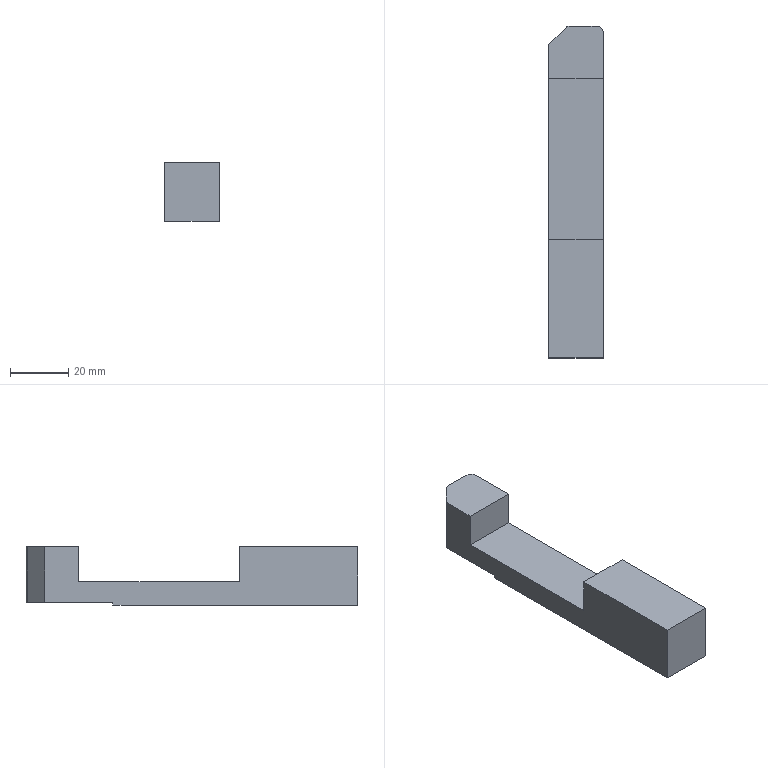Part | NX | features 20 2 | 1 solid | 15 faces | box 18.5 x 113.5 x 20 mm | volume 28823 mm3 | plane 13 | cylinder 2 | commonest cylinder face diameters 4 x2
STEP:
#1=CARTESIAN_POINT('',(316.699,-435.5,4.5));
#2=VERTEX_POINT('',#1);
#3=CARTESIAN_POINT('',(316.699,-490.5,4.5));
#4=VERTEX_POINT('',#3);
#5=CARTESIAN_POINT('',(316.699,-483.5,4.5));
#6=DIRECTION('',(0.,-1.,0.));
#7=VECTOR('',#6,1000.);
#8=LINE('',#5,#7);
#9=EDGE_CURVE('',#2,#4,#8,.T.);
#10=ORIENTED_EDGE('',*,*,#9,.T.);
#11=CARTESIAN_POINT('',(335.199,-490.5,4.5));
#12=VERTEX_POINT('',#11);
#13=CARTESIAN_POINT('',(297.899,-490.5,4.5));
#14=DIRECTION('',(-1.,0.,0.));
#15=VECTOR('',#14,1000.);
#16=LINE('',#13,#15);
#17=EDGE_CURVE('',#12,#4,#16,.T.);
#18=ORIENTED_EDGE('',*,*,#17,.F.);
#19=CARTESIAN_POINT('',(335.199,-435.5,4.5));
#20=VERTEX_POINT('',#19);
#21=CARTESIAN_POINT('',(335.199,-419.,4.5));
#22=DIRECTION('',(0.,1.,0.));
#23=VECTOR('',#22,1000.);
#24=LINE('',#21,#23);
#25=EDGE_CURVE('',#12,#20,#24,.T.);
#26=ORIENTED_EDGE('',*,*,#25,.T.);
#27=CARTESIAN_POINT('',(320.299,-435.5,4.5));
#28=DIRECTION('',(-1.,0.,0.));
#29=VECTOR('',#28,1000.);
#30=LINE('',#27,#29);
#31=EDGE_CURVE('',#20,#2,#30,.T.);
#32=ORIENTED_EDGE('',*,*,#31,.T.);
#33=EDGE_LOOP('',(#10,#18,#26,#32));
#34=FACE_BOUND('',#33,.T.);
#35=CARTESIAN_POINT('',(296.899,-343.,4.5));
#36=DIRECTION('',(0.,0.,1.));
#37=DIRECTION('',(1.,0.,0.));
#38=AXIS2_PLACEMENT_3D('',#35,#36,#37);
#39=PLANE('',#38);
#40=ADVANCED_FACE('',(#34),#39,.T.);
#41=CARTESIAN_POINT('',(316.699,-447.223,-2.5));
#42=VERTEX_POINT('',#41);
#43=CARTESIAN_POINT('',(316.699,-423.94,-2.5));
#44=VERTEX_POINT('',#43);
#45=CARTESIAN_POINT('',(316.699,-483.5,-2.5));
#46=DIRECTION('',(0.,1.,0.));
#47=VECTOR('',#46,1000.);
#48=LINE('',#45,#47);
#49=EDGE_CURVE('',#42,#44,#48,.T.);
#50=ORIENTED_EDGE('',*,*,#49,.F.);
#51=CARTESIAN_POINT('',(316.699,-447.223,-3.5));
#52=VERTEX_POINT('',#51);
#53=CARTESIAN_POINT('',(316.699,-447.223,-3.5));
#54=DIRECTION('',(0.,0.,1.));
#55=VECTOR('',#54,1000.);
#56=LINE('',#53,#55);
#57=EDGE_CURVE('',#52,#42,#56,.T.);
#58=ORIENTED_EDGE('',*,*,#57,.F.);
#59=CARTESIAN_POINT('',(316.699,-531.,-3.5));
#60=VERTEX_POINT('',#59);
#61=CARTESIAN_POINT('',(316.699,-483.5,-3.5));
#62=DIRECTION('',(0.,1.,0.));
#63=VECTOR('',#62,1000.);
#64=LINE('',#61,#63);
#65=EDGE_CURVE('',#60,#52,#64,.T.);
#66=ORIENTED_EDGE('',*,*,#65,.F.);
#67=CARTESIAN_POINT('',(316.699,-531.,16.5));
#68=VERTEX_POINT('',#67);
#69=CARTESIAN_POINT('',(316.699,-531.,-3.5));
#70=DIRECTION('',(0.,0.,1.));
#71=VECTOR('',#70,1000.);
#72=LINE('',#69,#71);
#73=EDGE_CURVE('',#60,#68,#72,.T.);
#74=ORIENTED_EDGE('',*,*,#73,.T.);
#75=CARTESIAN_POINT('',(316.699,-490.5,16.5));
#76=VERTEX_POINT('',#75);
#77=CARTESIAN_POINT('',(316.699,-453.,16.5));
#78=DIRECTION('',(0.,1.,0.));
#79=VECTOR('',#78,1000.);
#80=LINE('',#77,#79);
#81=EDGE_CURVE('',#68,#76,#80,.T.);
#82=ORIENTED_EDGE('',*,*,#81,.T.);
#83=CARTESIAN_POINT('',(316.699,-490.5,-3.5));
#84=DIRECTION('',(0.,0.,-1.));
#85=VECTOR('',#84,1000.);
#86=LINE('',#83,#85);
#87=EDGE_CURVE('',#76,#4,#86,.T.);
#88=ORIENTED_EDGE('',*,*,#87,.T.);
#89=ORIENTED_EDGE('',*,*,#9,.F.);
#90=CARTESIAN_POINT('',(316.699,-435.5,16.5));
#91=VERTEX_POINT('',#90);
#92=CARTESIAN_POINT('',(316.699,-435.5,22.5));
#93=DIRECTION('',(0.,0.,1.));
#94=VECTOR('',#93,1000.);
#95=LINE('',#92,#94);
#96=EDGE_CURVE('',#2,#91,#95,.T.);
#97=ORIENTED_EDGE('',*,*,#96,.T.);
#98=CARTESIAN_POINT('',(316.699,-423.94,16.5));
#99=VERTEX_POINT('',#98);
#100=CARTESIAN_POINT('',(316.699,-468.,16.5));
#101=DIRECTION('',(0.,1.,0.));
#102=VECTOR('',#101,1000.);
#103=LINE('',#100,#102);
#104=EDGE_CURVE('',#91,#99,#103,.T.);
#105=ORIENTED_EDGE('',*,*,#104,.T.);
#106=CARTESIAN_POINT('',(316.699,-423.94,-2.));
#107=DIRECTION('',(0.,0.,1.));
#108=VECTOR('',#107,1000.);
#109=LINE('',#106,#108);
#110=EDGE_CURVE('',#44,#99,#109,.T.);
#111=ORIENTED_EDGE('',*,*,#110,.F.);
#112=EDGE_LOOP('',(#50,#58,#66,#74,#82,#88,#89,#97,#105,#111));
#113=FACE_BOUND('',#112,.T.);
#114=CARTESIAN_POINT('',(316.699,-483.5,-3.5));
#115=DIRECTION('',(1.,0.,0.));
#116=DIRECTION('',(0.,1.,0.));
#117=AXIS2_PLACEMENT_3D('',#114,#115,#116);
#118=PLANE('',#117);
#119=ADVANCED_FACE('',(#113),#118,.F.);
#120=CARTESIAN_POINT('',(335.199,-447.223,-2.5));
#121=VERTEX_POINT('',#120);
#122=CARTESIAN_POINT('',(433.109,-447.223,-2.5));
#123=DIRECTION('',(-1.,0.,0.));
#124=VECTOR('',#123,1000.);
#125=LINE('',#122,#124);
#126=EDGE_CURVE('',#121,#42,#125,.T.);
#127=ORIENTED_EDGE('',*,*,#126,.T.);
#128=ORIENTED_EDGE('',*,*,#49,.T.);
#129=CARTESIAN_POINT('',(322.553,-418.086,-2.5));
#130=VERTEX_POINT('',#129);
#131=CARTESIAN_POINT('',(320.376,-420.263,-2.5));
#132=DIRECTION('',(0.7071,0.7071,0.));
#133=VECTOR('',#132,1000.);
#134=LINE('',#131,#133);
#135=EDGE_CURVE('',#44,#130,#134,.T.);
#136=ORIENTED_EDGE('',*,*,#135,.T.);
#137=CARTESIAN_POINT('',(323.967,-417.5,-2.5));
#138=VERTEX_POINT('',#137);
#139=CARTESIAN_POINT('',(323.967,-419.5,-2.5));
#140=DIRECTION('',(0.,0.,-1.));
#141=DIRECTION('',(-1.,0.,0.));
#142=AXIS2_PLACEMENT_3D('',#139,#140,#141);
#143=CIRCLE('',#142,2.);
#144=EDGE_CURVE('',#130,#138,#143,.T.);
#145=ORIENTED_EDGE('',*,*,#144,.T.);
#146=CARTESIAN_POINT('',(333.199,-417.5,-2.5));
#147=VERTEX_POINT('',#146);
#148=CARTESIAN_POINT('',(325.199,-417.5,-2.5));
#149=DIRECTION('',(1.,0.,0.));
#150=VECTOR('',#149,1000.);
#151=LINE('',#148,#150);
#152=EDGE_CURVE('',#138,#147,#151,.T.);
#153=ORIENTED_EDGE('',*,*,#152,.T.);
#154=CARTESIAN_POINT('',(335.199,-419.5,-2.5));
#155=VERTEX_POINT('',#154);
#156=CARTESIAN_POINT('',(333.199,-419.5,-2.5));
#157=DIRECTION('',(0.,0.,-1.));
#158=DIRECTION('',(-1.,0.,0.));
#159=AXIS2_PLACEMENT_3D('',#156,#157,#158);
#160=CIRCLE('',#159,2.);
#161=EDGE_CURVE('',#147,#155,#160,.T.);
#162=ORIENTED_EDGE('',*,*,#161,.T.);
#163=CARTESIAN_POINT('',(335.199,-419.,-2.5));
#164=DIRECTION('',(0.,-1.,0.));
#165=VECTOR('',#164,1000.);
#166=LINE('',#163,#165);
#167=EDGE_CURVE('',#155,#121,#166,.T.);
#168=ORIENTED_EDGE('',*,*,#167,.T.);
#169=EDGE_LOOP('',(#127,#128,#136,#145,#153,#162,#168));
#170=FACE_BOUND('',#169,.T.);
#171=CARTESIAN_POINT('',(325.199,-419.,-2.5));
#172=DIRECTION('',(0.,0.,-1.));
#173=DIRECTION('',(-1.,0.,0.));
#174=AXIS2_PLACEMENT_3D('',#171,#172,#173);
#175=PLANE('',#174);
#176=ADVANCED_FACE('',(#170),#175,.T.);
#177=ORIENTED_EDGE('',*,*,#25,.F.);
#178=CARTESIAN_POINT('',(335.199,-490.5,16.5));
#179=VERTEX_POINT('',#178);
#180=CARTESIAN_POINT('',(335.199,-490.5,-3.5));
#181=DIRECTION('',(0.,0.,1.));
#182=VECTOR('',#181,1000.);
#183=LINE('',#180,#182);
#184=EDGE_CURVE('',#12,#179,#183,.T.);
#185=ORIENTED_EDGE('',*,*,#184,.T.);
#186=CARTESIAN_POINT('',(335.199,-531.,16.5));
#187=VERTEX_POINT('',#186);
#188=CARTESIAN_POINT('',(335.199,-453.,16.5));
#189=DIRECTION('',(0.,-1.,0.));
#190=VECTOR('',#189,1000.);
#191=LINE('',#188,#190);
#192=EDGE_CURVE('',#179,#187,#191,.T.);
#193=ORIENTED_EDGE('',*,*,#192,.T.);
#194=CARTESIAN_POINT('',(335.199,-531.,-3.5));
#195=VERTEX_POINT('',#194);
#196=CARTESIAN_POINT('',(335.199,-531.,-43.5));
#197=DIRECTION('',(0.,0.,1.));
#198=VECTOR('',#197,1000.);
#199=LINE('',#196,#198);
#200=EDGE_CURVE('',#195,#187,#199,.T.);
#201=ORIENTED_EDGE('',*,*,#200,.F.);
#202=CARTESIAN_POINT('',(335.199,-447.223,-3.5));
#203=VERTEX_POINT('',#202);
#204=CARTESIAN_POINT('',(335.199,-419.,-3.5));
#205=DIRECTION('',(0.,-1.,0.));
#206=VECTOR('',#205,1000.);
#207=LINE('',#204,#206);
#208=EDGE_CURVE('',#203,#195,#207,.T.);
#209=ORIENTED_EDGE('',*,*,#208,.F.);
#210=CARTESIAN_POINT('',(335.199,-447.223,-21.));
#211=DIRECTION('',(0.,0.,1.));
#212=VECTOR('',#211,1000.);
#213=LINE('',#210,#212);
#214=EDGE_CURVE('',#203,#121,#213,.T.);
#215=ORIENTED_EDGE('',*,*,#214,.T.);
#216=ORIENTED_EDGE('',*,*,#167,.F.);
#217=CARTESIAN_POINT('',(335.199,-419.5,16.5));
#218=VERTEX_POINT('',#217);
#219=CARTESIAN_POINT('',(335.199,-419.5,-3.5));
#220=DIRECTION('',(0.,0.,1.));
#221=VECTOR('',#220,1000.);
#222=LINE('',#219,#221);
#223=EDGE_CURVE('',#155,#218,#222,.T.);
#224=ORIENTED_EDGE('',*,*,#223,.T.);
#225=CARTESIAN_POINT('',(335.199,-435.5,16.5));
#226=VERTEX_POINT('',#225);
#227=CARTESIAN_POINT('',(335.199,-468.,16.5));
#228=DIRECTION('',(0.,-1.,0.));
#229=VECTOR('',#228,1000.);
#230=LINE('',#227,#229);
#231=EDGE_CURVE('',#218,#226,#230,.T.);
#232=ORIENTED_EDGE('',*,*,#231,.T.);
#233=CARTESIAN_POINT('',(335.199,-435.5,22.5));
#234=DIRECTION('',(0.,0.,-1.));
#235=VECTOR('',#234,1000.);
#236=LINE('',#233,#235);
#237=EDGE_CURVE('',#226,#20,#236,.T.);
#238=ORIENTED_EDGE('',*,*,#237,.T.);
#239=EDGE_LOOP('',(#177,#185,#193,#201,#209,#215,#216,#224,#232,#238));
#240=FACE_BOUND('',#239,.T.);
#241=CARTESIAN_POINT('',(335.199,-419.,-3.5));
#242=DIRECTION('',(-1.,0.,0.));
#243=DIRECTION('',(0.,0.,1.));
#244=AXIS2_PLACEMENT_3D('',#241,#242,#243);
#245=PLANE('',#244);
#246=ADVANCED_FACE('',(#240),#245,.F.);
#247=CARTESIAN_POINT('',(305.899,-435.5,16.5));
#248=DIRECTION('',(1.,0.,0.));
#249=VECTOR('',#248,1000.);
#250=LINE('',#247,#249);
#251=EDGE_CURVE('',#91,#226,#250,.T.);
#252=ORIENTED_EDGE('',*,*,#251,.F.);
#253=ORIENTED_EDGE('',*,*,#96,.F.);
#254=ORIENTED_EDGE('',*,*,#31,.F.);
#255=ORIENTED_EDGE('',*,*,#237,.F.);
#256=EDGE_LOOP('',(#252,#253,#254,#255));
#257=FACE_BOUND('',#256,.T.);
#258=CARTESIAN_POINT('',(320.299,-435.5,22.5));
#259=DIRECTION('',(0.,-1.,0.));
#260=DIRECTION('',(0.,0.,1.));
#261=AXIS2_PLACEMENT_3D('',#258,#259,#260);
#262=PLANE('',#261);
#263=ADVANCED_FACE('',(#257),#262,.T.);
#264=ORIENTED_EDGE('',*,*,#135,.F.);
#265=ORIENTED_EDGE('',*,*,#110,.T.);
#266=CARTESIAN_POINT('',(322.553,-418.086,16.5));
#267=VERTEX_POINT('',#266);
#268=CARTESIAN_POINT('',(289.269,-451.37,16.5));
#269=DIRECTION('',(0.7071,0.7071,0.));
#270=VECTOR('',#269,1000.);
#271=LINE('',#268,#270);
#272=EDGE_CURVE('',#99,#267,#271,.T.);
#273=ORIENTED_EDGE('',*,*,#272,.T.);
#274=CARTESIAN_POINT('',(322.553,-418.086,4.5));
#275=DIRECTION('',(0.,0.,-1.));
#276=VECTOR('',#275,1000.);
#277=LINE('',#274,#276);
#278=EDGE_CURVE('',#267,#130,#277,.T.);
#279=ORIENTED_EDGE('',*,*,#278,.T.);
#280=EDGE_LOOP('',(#264,#265,#273,#279));
#281=FACE_BOUND('',#280,.T.);
#282=CARTESIAN_POINT('',(320.376,-420.263,-2.));
#283=DIRECTION('',(0.7071,-0.7071,0.));
#284=DIRECTION('',(0.7071,0.7071,0.));
#285=AXIS2_PLACEMENT_3D('',#282,#283,#284);
#286=PLANE('',#285);
#287=ADVANCED_FACE('',(#281),#286,.F.);
#288=CARTESIAN_POINT('',(323.967,-417.5,16.5));
#289=VERTEX_POINT('',#288);
#290=CARTESIAN_POINT('',(333.199,-417.5,16.5));
#291=VERTEX_POINT('',#290);
#292=CARTESIAN_POINT('',(301.424,-417.5,16.5));
#293=DIRECTION('',(1.,0.,0.));
#294=VECTOR('',#293,1000.);
#295=LINE('',#292,#294);
#296=EDGE_CURVE('',#289,#291,#295,.T.);
#297=ORIENTED_EDGE('',*,*,#296,.F.);
#298=CARTESIAN_POINT('',(323.967,-419.5,16.5));
#299=DIRECTION('',(0.,0.,1.));
#300=DIRECTION('',(1.,0.,0.));
#301=AXIS2_PLACEMENT_3D('',#298,#299,#300);
#302=CIRCLE('',#301,2.);
#303=EDGE_CURVE('',#289,#267,#302,.T.);
#304=ORIENTED_EDGE('',*,*,#303,.T.);
#305=ORIENTED_EDGE('',*,*,#272,.F.);
#306=ORIENTED_EDGE('',*,*,#104,.F.);
#307=ORIENTED_EDGE('',*,*,#251,.T.);
#308=ORIENTED_EDGE('',*,*,#231,.F.);
#309=CARTESIAN_POINT('',(333.199,-419.5,16.5));
#310=DIRECTION('',(0.,0.,1.));
#311=DIRECTION('',(1.,0.,0.));
#312=AXIS2_PLACEMENT_3D('',#309,#310,#311);
#313=CIRCLE('',#312,2.);
#314=EDGE_CURVE('',#218,#291,#313,.T.);
#315=ORIENTED_EDGE('',*,*,#314,.T.);
#316=EDGE_LOOP('',(#297,#304,#305,#306,#307,#308,#315));
#317=FACE_BOUND('',#316,.T.);
#318=CARTESIAN_POINT('',(305.899,-468.,16.5));
#319=DIRECTION('',(0.,0.,1.));
#320=DIRECTION('',(1.,0.,0.));
#321=AXIS2_PLACEMENT_3D('',#318,#319,#320);
#322=PLANE('',#321);
#323=ADVANCED_FACE('',(#317),#322,.T.);
#324=ORIENTED_EDGE('',*,*,#152,.F.);
#325=CARTESIAN_POINT('',(323.967,-417.5,4.5));
#326=DIRECTION('',(0.,0.,1.));
#327=VECTOR('',#326,1000.);
#328=LINE('',#325,#327);
#329=EDGE_CURVE('',#138,#289,#328,.T.);
#330=ORIENTED_EDGE('',*,*,#329,.T.);
#331=ORIENTED_EDGE('',*,*,#296,.T.);
#332=CARTESIAN_POINT('',(333.199,-417.5,-3.5));
#333=DIRECTION('',(0.,0.,-1.));
#334=VECTOR('',#333,1000.);
#335=LINE('',#332,#334);
#336=EDGE_CURVE('',#291,#147,#335,.T.);
#337=ORIENTED_EDGE('',*,*,#336,.T.);
#338=EDGE_LOOP('',(#324,#330,#331,#337));
#339=FACE_BOUND('',#338,.T.);
#340=CARTESIAN_POINT('',(301.424,-417.5,4.5));
#341=DIRECTION('',(0.,1.,0.));
#342=DIRECTION('',(0.,0.,-1.));
#343=AXIS2_PLACEMENT_3D('',#340,#341,#342);
#344=PLANE('',#343);
#345=ADVANCED_FACE('',(#339),#344,.T.);
#346=ORIENTED_EDGE('',*,*,#303,.F.);
#347=ORIENTED_EDGE('',*,*,#329,.F.);
#348=ORIENTED_EDGE('',*,*,#144,.F.);
#349=ORIENTED_EDGE('',*,*,#278,.F.);
#350=EDGE_LOOP('',(#346,#347,#348,#349));
#351=FACE_BOUND('',#350,.T.);
#352=CARTESIAN_POINT('',(323.967,-419.5,4.5));
#353=DIRECTION('',(0.,0.,-1.));
#354=DIRECTION('',(-1.,0.,0.));
#355=AXIS2_PLACEMENT_3D('',#352,#353,#354);
#356=CYLINDRICAL_SURFACE('',#355,2.);
#357=ADVANCED_FACE('',(#351),#356,.T.);
#358=ORIENTED_EDGE('',*,*,#314,.F.);
#359=ORIENTED_EDGE('',*,*,#223,.F.);
#360=ORIENTED_EDGE('',*,*,#161,.F.);
#361=ORIENTED_EDGE('',*,*,#336,.F.);
#362=EDGE_LOOP('',(#358,#359,#360,#361));
#363=FACE_BOUND('',#362,.T.);
#364=CARTESIAN_POINT('',(333.199,-419.5,-3.5));
#365=DIRECTION('',(0.,0.,-1.));
#366=DIRECTION('',(-1.,0.,0.));
#367=AXIS2_PLACEMENT_3D('',#364,#365,#366);
#368=CYLINDRICAL_SURFACE('',#367,2.);
#369=ADVANCED_FACE('',(#363),#368,.T.);
#370=ORIENTED_EDGE('',*,*,#126,.F.);
#371=ORIENTED_EDGE('',*,*,#214,.F.);
#372=CARTESIAN_POINT('',(325.199,-447.223,-3.5));
#373=DIRECTION('',(1.,0.,0.));
#374=VECTOR('',#373,1000.);
#375=LINE('',#372,#374);
#376=EDGE_CURVE('',#52,#203,#375,.T.);
#377=ORIENTED_EDGE('',*,*,#376,.F.);
#378=ORIENTED_EDGE('',*,*,#57,.T.);
#379=EDGE_LOOP('',(#370,#371,#377,#378));
#380=FACE_BOUND('',#379,.T.);
#381=CARTESIAN_POINT('',(433.109,-447.223,-21.));
#382=DIRECTION('',(0.,1.,0.));
#383=DIRECTION('',(0.,0.,-1.));
#384=AXIS2_PLACEMENT_3D('',#381,#382,#383);
#385=PLANE('',#384);
#386=ADVANCED_FACE('',(#380),#385,.T.);
#387=CARTESIAN_POINT('',(305.899,-531.,16.5));
#388=DIRECTION('',(-1.,0.,0.));
#389=VECTOR('',#388,1000.);
#390=LINE('',#387,#389);
#391=EDGE_CURVE('',#187,#68,#390,.T.);
#392=ORIENTED_EDGE('',*,*,#391,.T.);
#393=ORIENTED_EDGE('',*,*,#73,.F.);
#394=CARTESIAN_POINT('',(508.899,-531.,-3.5));
#395=DIRECTION('',(-1.,0.,0.));
#396=VECTOR('',#395,1000.);
#397=LINE('',#394,#396);
#398=EDGE_CURVE('',#195,#60,#397,.T.);
#399=ORIENTED_EDGE('',*,*,#398,.F.);
#400=ORIENTED_EDGE('',*,*,#200,.T.);
#401=EDGE_LOOP('',(#392,#393,#399,#400));
#402=FACE_BOUND('',#401,.T.);
#403=CARTESIAN_POINT('',(508.899,-531.,-43.5));
#404=DIRECTION('',(0.,1.,0.));
#405=DIRECTION('',(0.,0.,1.));
#406=AXIS2_PLACEMENT_3D('',#403,#404,#405);
#407=PLANE('',#406);
#408=ADVANCED_FACE('',(#402),#407,.F.);
#409=ORIENTED_EDGE('',*,*,#192,.F.);
#410=CARTESIAN_POINT('',(297.899,-490.5,16.5));
#411=DIRECTION('',(-1.,0.,0.));
#412=VECTOR('',#411,1000.);
#413=LINE('',#410,#412);
#414=EDGE_CURVE('',#179,#76,#413,.T.);
#415=ORIENTED_EDGE('',*,*,#414,.T.);
#416=ORIENTED_EDGE('',*,*,#81,.F.);
#417=ORIENTED_EDGE('',*,*,#391,.F.);
#418=EDGE_LOOP('',(#409,#415,#416,#417));
#419=FACE_BOUND('',#418,.T.);
#420=CARTESIAN_POINT('',(305.899,-453.,16.5));
#421=DIRECTION('',(0.,0.,1.));
#422=DIRECTION('',(1.,0.,0.));
#423=AXIS2_PLACEMENT_3D('',#420,#421,#422);
#424=PLANE('',#423);
#425=ADVANCED_FACE('',(#419),#424,.T.);
#426=ORIENTED_EDGE('',*,*,#17,.T.);
#427=ORIENTED_EDGE('',*,*,#87,.F.);
#428=ORIENTED_EDGE('',*,*,#414,.F.);
#429=ORIENTED_EDGE('',*,*,#184,.F.);
#430=EDGE_LOOP('',(#426,#427,#428,#429));
#431=FACE_BOUND('',#430,.T.);
#432=CARTESIAN_POINT('',(297.899,-490.5,8.5));
#433=DIRECTION('',(0.,-1.,0.));
#434=DIRECTION('',(0.,0.,-1.));
#435=AXIS2_PLACEMENT_3D('',#432,#433,#434);
#436=PLANE('',#435);
#437=ADVANCED_FACE('',(#431),#436,.F.);
#438=ORIENTED_EDGE('',*,*,#65,.T.);
#439=ORIENTED_EDGE('',*,*,#376,.T.);
#440=ORIENTED_EDGE('',*,*,#208,.T.);
#441=ORIENTED_EDGE('',*,*,#398,.T.);
#442=EDGE_LOOP('',(#438,#439,#440,#441));
#443=FACE_BOUND('',#442,.T.);
#444=CARTESIAN_POINT('',(325.199,-419.,-3.5));
#445=DIRECTION('',(0.,0.,-1.));
#446=DIRECTION('',(-1.,0.,0.));
#447=AXIS2_PLACEMENT_3D('',#444,#445,#446);
#448=PLANE('',#447);
#449=ADVANCED_FACE('',(#443),#448,.T.);
#450=CLOSED_SHELL('',(#40,#119,#176,#246,#263,#287,#323,#345,#357,#369,#386,#408,#425,#437,#449));
#451=MANIFOLD_SOLID_BREP('',#450);
#452=(LENGTH_UNIT()NAMED_UNIT(*)SI_UNIT(.MILLI.,.METRE.));
#453=UNCERTAINTY_MEASURE_WITH_UNIT(LENGTH_MEASURE(0.00001),#452,'','');
#454=(NAMED_UNIT(*)PLANE_ANGLE_UNIT()SI_UNIT($,.RADIAN.));
#455=(NAMED_UNIT(*)SI_UNIT($,.STERADIAN.)SOLID_ANGLE_UNIT());
#456=(GEOMETRIC_REPRESENTATION_CONTEXT(3)GLOBAL_UNCERTAINTY_ASSIGNED_CONTEXT((#453))GLOBAL_UNIT_ASSIGNED_CONTEXT((#452,#454,#455))REPRESENTATION_CONTEXT('',''));
#457=ADVANCED_BREP_SHAPE_REPRESENTATION('',(#451),#456);